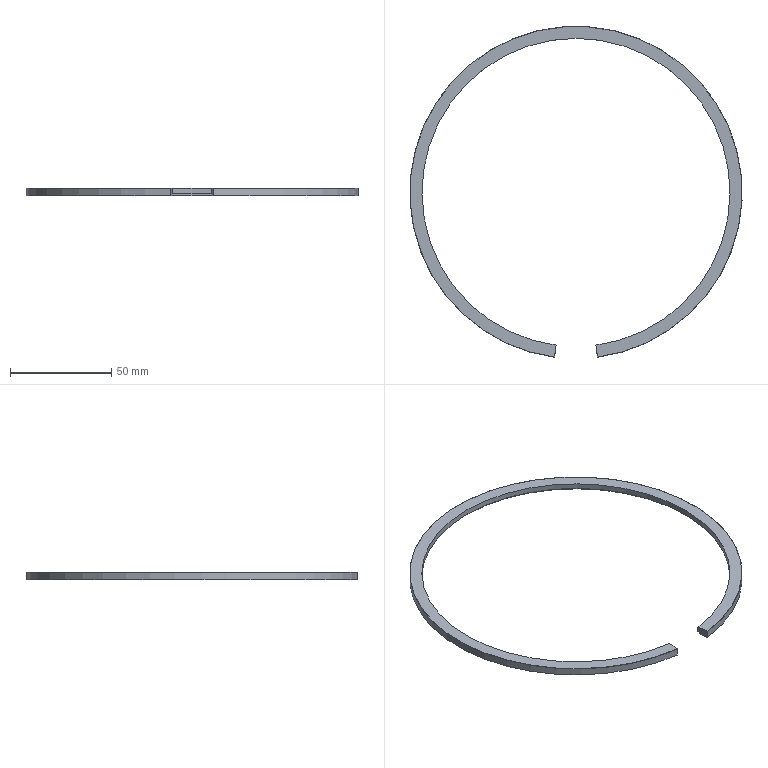Part | NX | features DATUM_CSYS 3, EXTRUDE 2, SKETCH 2, BLEND 1, TEXT 1 | 1 solid | 9 faces | box 164 x 163.314 x 3.7 mm | volume 10104 mm3 | plane 5 | cylinder 3 | torus 1 | commonest cylinder face diameters 152 x1 154 x1 164 x1
STEP:
#1=CARTESIAN_POINT('',(-10.571,-81.215,3.7));
#2=VERTEX_POINT('',#1);
#3=CARTESIAN_POINT('',(-9.81,-75.364,3.7));
#4=VERTEX_POINT('',#3);
#5=CARTESIAN_POINT('',(-10.584,-81.314,3.7));
#6=DIRECTION('',(0.1291,0.9916,0.));
#7=VECTOR('',#6,1000.);
#8=LINE('',#5,#7);
#9=EDGE_CURVE('',#2,#4,#8,.T.);
#10=ORIENTED_EDGE('',*,*,#9,.F.);
#11=CARTESIAN_POINT('',(-10.584,-81.314,3.6));
#12=VERTEX_POINT('',#11);
#13=CARTESIAN_POINT('',(-10.571,-81.215,3.6));
#14=DIRECTION('',(-0.9916,0.1291,0.));
#15=DIRECTION('',(-0.1291,-0.9916,0.));
#16=AXIS2_PLACEMENT_3D('',#13,#14,#15);
#17=CIRCLE('',#16,0.1);
#18=EDGE_CURVE('',#2,#12,#17,.F.);
#19=ORIENTED_EDGE('',*,*,#18,.T.);
#20=CARTESIAN_POINT('',(-10.584,-81.314,0.));
#21=VERTEX_POINT('',#20);
#22=CARTESIAN_POINT('',(-10.584,-81.314,3.7));
#23=DIRECTION('',(0.,0.,-1.));
#24=VECTOR('',#23,1000.);
#25=LINE('',#22,#24);
#26=EDGE_CURVE('',#12,#21,#25,.T.);
#27=ORIENTED_EDGE('',*,*,#26,.T.);
#28=CARTESIAN_POINT('',(-9.939,-76.356,0.));
#29=VERTEX_POINT('',#28);
#30=CARTESIAN_POINT('',(-10.584,-81.314,0.));
#31=DIRECTION('',(0.1291,0.9916,0.));
#32=VECTOR('',#31,1000.);
#33=LINE('',#30,#32);
#34=EDGE_CURVE('',#21,#29,#33,.T.);
#35=ORIENTED_EDGE('',*,*,#34,.T.);
#36=CARTESIAN_POINT('',(-9.939,-76.356,1.));
#37=VERTEX_POINT('',#36);
#38=CARTESIAN_POINT('',(-9.939,-76.356,1.));
#39=DIRECTION('',(0.,0.,-1.));
#40=VECTOR('',#39,1000.);
#41=LINE('',#38,#40);
#42=EDGE_CURVE('',#37,#29,#41,.T.);
#43=ORIENTED_EDGE('',*,*,#42,.F.);
#44=CARTESIAN_POINT('',(-9.81,-75.364,1.));
#45=VERTEX_POINT('',#44);
#46=CARTESIAN_POINT('',(-9.81,-75.364,1.));
#47=DIRECTION('',(-0.1291,-0.9916,0.));
#48=VECTOR('',#47,1000.);
#49=LINE('',#46,#48);
#50=EDGE_CURVE('',#45,#37,#49,.T.);
#51=ORIENTED_EDGE('',*,*,#50,.F.);
#52=CARTESIAN_POINT('',(-9.81,-75.364,3.7));
#53=DIRECTION('',(0.,0.,-1.));
#54=VECTOR('',#53,1000.);
#55=LINE('',#52,#54);
#56=EDGE_CURVE('',#4,#45,#55,.T.);
#57=ORIENTED_EDGE('',*,*,#56,.F.);
#58=EDGE_LOOP('',(#10,#19,#27,#35,#43,#51,#57));
#59=FACE_BOUND('',#58,.T.);
#60=CARTESIAN_POINT('',(-10.584,-81.314,3.7));
#61=DIRECTION('',(-0.9916,0.1291,0.));
#62=DIRECTION('',(-0.1291,-0.9916,0.));
#63=AXIS2_PLACEMENT_3D('',#60,#61,#62);
#64=PLANE('',#63);
#65=ADVANCED_FACE('',(#59),#64,.F.);
#66=CARTESIAN_POINT('',(9.81,-75.364,1.));
#67=VERTEX_POINT('',#66);
#68=CARTESIAN_POINT('',(0.,0.,1.));
#69=DIRECTION('',(0.,0.,1.));
#70=DIRECTION('',(1.,0.,0.));
#71=AXIS2_PLACEMENT_3D('',#68,#69,#70);
#72=CIRCLE('',#71,76.);
#73=EDGE_CURVE('',#67,#45,#72,.T.);
#74=ORIENTED_EDGE('',*,*,#73,.F.);
#75=CARTESIAN_POINT('',(9.81,-75.364,3.7));
#76=VERTEX_POINT('',#75);
#77=CARTESIAN_POINT('',(9.81,-75.364,3.7));
#78=DIRECTION('',(0.,0.,-1.));
#79=VECTOR('',#78,1000.);
#80=LINE('',#77,#79);
#81=EDGE_CURVE('',#76,#67,#80,.T.);
#82=ORIENTED_EDGE('',*,*,#81,.F.);
#83=CARTESIAN_POINT('',(0.,0.,3.7));
#84=DIRECTION('',(0.,0.,-1.));
#85=DIRECTION('',(1.,0.,0.));
#86=AXIS2_PLACEMENT_3D('',#83,#84,#85);
#87=CIRCLE('',#86,76.);
#88=EDGE_CURVE('',#4,#76,#87,.T.);
#89=ORIENTED_EDGE('',*,*,#88,.F.);
#90=ORIENTED_EDGE('',*,*,#56,.T.);
#91=EDGE_LOOP('',(#74,#82,#89,#90));
#92=FACE_BOUND('',#91,.T.);
#93=CARTESIAN_POINT('',(0.,0.,3.7));
#94=DIRECTION('',(0.,0.,-1.));
#95=DIRECTION('',(-1.,0.,0.));
#96=AXIS2_PLACEMENT_3D('',#93,#94,#95);
#97=CYLINDRICAL_SURFACE('',#96,76.);
#98=ADVANCED_FACE('',(#92),#97,.F.);
#99=CARTESIAN_POINT('',(9.939,-76.356,0.));
#100=VERTEX_POINT('',#99);
#101=CARTESIAN_POINT('',(0.,0.,0.));
#102=DIRECTION('',(0.,0.,-1.));
#103=DIRECTION('',(1.,0.,0.));
#104=AXIS2_PLACEMENT_3D('',#101,#102,#103);
#105=CIRCLE('',#104,77.);
#106=EDGE_CURVE('',#29,#100,#105,.T.);
#107=ORIENTED_EDGE('',*,*,#106,.F.);
#108=ORIENTED_EDGE('',*,*,#34,.F.);
#109=CARTESIAN_POINT('',(10.584,-81.314,0.));
#110=VERTEX_POINT('',#109);
#111=CARTESIAN_POINT('',(0.,0.,0.));
#112=DIRECTION('',(0.,0.,1.));
#113=DIRECTION('',(1.,0.,0.));
#114=AXIS2_PLACEMENT_3D('',#111,#112,#113);
#115=CIRCLE('',#114,82.);
#116=EDGE_CURVE('',#110,#21,#115,.T.);
#117=ORIENTED_EDGE('',*,*,#116,.F.);
#118=CARTESIAN_POINT('',(9.81,-75.364,0.));
#119=DIRECTION('',(0.1291,-0.9916,0.));
#120=VECTOR('',#119,1000.);
#121=LINE('',#118,#120);
#122=EDGE_CURVE('',#100,#110,#121,.T.);
#123=ORIENTED_EDGE('',*,*,#122,.F.);
#124=EDGE_LOOP('',(#107,#108,#117,#123));
#125=FACE_BOUND('',#124,.T.);
#126=CARTESIAN_POINT('',(0.,0.,0.));
#127=DIRECTION('',(0.,0.,1.));
#128=DIRECTION('',(1.,0.,0.));
#129=AXIS2_PLACEMENT_3D('',#126,#127,#128);
#130=PLANE('',#129);
#131=ADVANCED_FACE('',(#125),#130,.F.);
#132=ORIENTED_EDGE('',*,*,#26,.F.);
#133=CARTESIAN_POINT('',(10.584,-81.314,3.6));
#134=VERTEX_POINT('',#133);
#135=CARTESIAN_POINT('',(0.,0.,3.6));
#136=DIRECTION('',(0.,0.,1.));
#137=DIRECTION('',(1.,0.,0.));
#138=AXIS2_PLACEMENT_3D('',#135,#136,#137);
#139=CIRCLE('',#138,82.);
#140=EDGE_CURVE('',#12,#134,#139,.F.);
#141=ORIENTED_EDGE('',*,*,#140,.T.);
#142=CARTESIAN_POINT('',(10.584,-81.314,3.7));
#143=DIRECTION('',(0.,0.,-1.));
#144=VECTOR('',#143,1000.);
#145=LINE('',#142,#144);
#146=EDGE_CURVE('',#134,#110,#145,.T.);
#147=ORIENTED_EDGE('',*,*,#146,.T.);
#148=ORIENTED_EDGE('',*,*,#116,.T.);
#149=EDGE_LOOP('',(#132,#141,#147,#148));
#150=FACE_BOUND('',#149,.T.);
#151=CARTESIAN_POINT('',(0.,0.,3.7));
#152=DIRECTION('',(0.,0.,-1.));
#153=DIRECTION('',(-1.,0.,0.));
#154=AXIS2_PLACEMENT_3D('',#151,#152,#153);
#155=CYLINDRICAL_SURFACE('',#154,82.);
#156=ADVANCED_FACE('',(#150),#155,.T.);
#157=ORIENTED_EDGE('',*,*,#146,.F.);
#158=CARTESIAN_POINT('',(10.571,-81.215,3.7));
#159=VERTEX_POINT('',#158);
#160=CARTESIAN_POINT('',(10.571,-81.215,3.6));
#161=DIRECTION('',(0.9916,0.1291,0.));
#162=DIRECTION('',(-0.1291,0.9916,0.));
#163=AXIS2_PLACEMENT_3D('',#160,#161,#162);
#164=CIRCLE('',#163,0.1);
#165=EDGE_CURVE('',#134,#159,#164,.F.);
#166=ORIENTED_EDGE('',*,*,#165,.T.);
#167=CARTESIAN_POINT('',(9.81,-75.364,3.7));
#168=DIRECTION('',(0.1291,-0.9916,0.));
#169=VECTOR('',#168,1000.);
#170=LINE('',#167,#169);
#171=EDGE_CURVE('',#76,#159,#170,.T.);
#172=ORIENTED_EDGE('',*,*,#171,.F.);
#173=ORIENTED_EDGE('',*,*,#81,.T.);
#174=CARTESIAN_POINT('',(9.939,-76.356,1.));
#175=VERTEX_POINT('',#174);
#176=CARTESIAN_POINT('',(9.939,-76.356,1.));
#177=DIRECTION('',(-0.1291,0.9916,0.));
#178=VECTOR('',#177,1000.);
#179=LINE('',#176,#178);
#180=EDGE_CURVE('',#175,#67,#179,.T.);
#181=ORIENTED_EDGE('',*,*,#180,.F.);
#182=CARTESIAN_POINT('',(9.939,-76.356,1.));
#183=DIRECTION('',(0.,0.,-1.));
#184=VECTOR('',#183,1000.);
#185=LINE('',#182,#184);
#186=EDGE_CURVE('',#175,#100,#185,.T.);
#187=ORIENTED_EDGE('',*,*,#186,.T.);
#188=ORIENTED_EDGE('',*,*,#122,.T.);
#189=EDGE_LOOP('',(#157,#166,#172,#173,#181,#187,#188));
#190=FACE_BOUND('',#189,.T.);
#191=CARTESIAN_POINT('',(9.81,-75.364,3.7));
#192=DIRECTION('',(0.9916,0.1291,0.));
#193=DIRECTION('',(-0.1291,0.9916,0.));
#194=AXIS2_PLACEMENT_3D('',#191,#192,#193);
#195=PLANE('',#194);
#196=ADVANCED_FACE('',(#190),#195,.F.);
#197=ORIENTED_EDGE('',*,*,#171,.T.);
#198=CARTESIAN_POINT('',(0.,0.,3.7));
#199=DIRECTION('',(0.,0.,1.));
#200=DIRECTION('',(1.,0.,0.));
#201=AXIS2_PLACEMENT_3D('',#198,#199,#200);
#202=CIRCLE('',#201,81.9);
#203=EDGE_CURVE('',#159,#2,#202,.T.);
#204=ORIENTED_EDGE('',*,*,#203,.T.);
#205=ORIENTED_EDGE('',*,*,#9,.T.);
#206=ORIENTED_EDGE('',*,*,#88,.T.);
#207=EDGE_LOOP('',(#197,#204,#205,#206));
#208=FACE_BOUND('',#207,.T.);
#209=CARTESIAN_POINT('',(0.,0.,3.7));
#210=DIRECTION('',(0.,0.,1.));
#211=DIRECTION('',(1.,0.,0.));
#212=AXIS2_PLACEMENT_3D('',#209,#210,#211);
#213=PLANE('',#212);
#214=ADVANCED_FACE('',(#208),#213,.T.);
#215=ORIENTED_EDGE('',*,*,#106,.T.);
#216=ORIENTED_EDGE('',*,*,#186,.F.);
#217=CARTESIAN_POINT('',(0.,0.,1.));
#218=DIRECTION('',(0.,0.,-1.));
#219=DIRECTION('',(1.,0.,0.));
#220=AXIS2_PLACEMENT_3D('',#217,#218,#219);
#221=CIRCLE('',#220,77.);
#222=EDGE_CURVE('',#175,#37,#221,.F.);
#223=ORIENTED_EDGE('',*,*,#222,.T.);
#224=ORIENTED_EDGE('',*,*,#42,.T.);
#225=EDGE_LOOP('',(#215,#216,#223,#224));
#226=FACE_BOUND('',#225,.T.);
#227=CARTESIAN_POINT('',(0.,0.,1.));
#228=DIRECTION('',(0.,0.,-1.));
#229=DIRECTION('',(-1.,0.,0.));
#230=AXIS2_PLACEMENT_3D('',#227,#228,#229);
#231=CYLINDRICAL_SURFACE('',#230,77.);
#232=ADVANCED_FACE('',(#226),#231,.F.);
#233=ORIENTED_EDGE('',*,*,#222,.F.);
#234=ORIENTED_EDGE('',*,*,#180,.T.);
#235=ORIENTED_EDGE('',*,*,#73,.T.);
#236=ORIENTED_EDGE('',*,*,#50,.T.);
#237=EDGE_LOOP('',(#233,#234,#235,#236));
#238=FACE_BOUND('',#237,.T.);
#239=CARTESIAN_POINT('',(0.,0.,1.));
#240=DIRECTION('',(0.,0.,-1.));
#241=DIRECTION('',(-1.,0.,0.));
#242=AXIS2_PLACEMENT_3D('',#239,#240,#241);
#243=PLANE('',#242);
#244=ADVANCED_FACE('',(#238),#243,.T.);
#245=ORIENTED_EDGE('',*,*,#165,.F.);
#246=ORIENTED_EDGE('',*,*,#140,.F.);
#247=ORIENTED_EDGE('',*,*,#18,.F.);
#248=ORIENTED_EDGE('',*,*,#203,.F.);
#249=EDGE_LOOP('',(#245,#246,#247,#248));
#250=FACE_BOUND('',#249,.T.);
#251=CARTESIAN_POINT('',(0.,0.,3.6));
#252=DIRECTION('',(0.,0.,1.));
#253=DIRECTION('',(1.,0.,0.));
#254=AXIS2_PLACEMENT_3D('',#251,#252,#253);
#255=TOROIDAL_SURFACE('',#254,81.9,0.1);
#256=ADVANCED_FACE('',(#250),#255,.T.);
#257=CLOSED_SHELL('',(#65,#98,#131,#156,#196,#214,#232,#244,#256));
#258=MANIFOLD_SOLID_BREP('',#257);
#259=(LENGTH_UNIT()NAMED_UNIT(*)SI_UNIT(.MILLI.,.METRE.));
#260=UNCERTAINTY_MEASURE_WITH_UNIT(LENGTH_MEASURE(0.00001),#259,'','');
#261=(NAMED_UNIT(*)PLANE_ANGLE_UNIT()SI_UNIT($,.RADIAN.));
#262=(NAMED_UNIT(*)SI_UNIT($,.STERADIAN.)SOLID_ANGLE_UNIT());
#263=(GEOMETRIC_REPRESENTATION_CONTEXT(3)GLOBAL_UNCERTAINTY_ASSIGNED_CONTEXT((#260))GLOBAL_UNIT_ASSIGNED_CONTEXT((#259,#261,#262))REPRESENTATION_CONTEXT('',''));
#264=ADVANCED_BREP_SHAPE_REPRESENTATION('',(#258),#263);